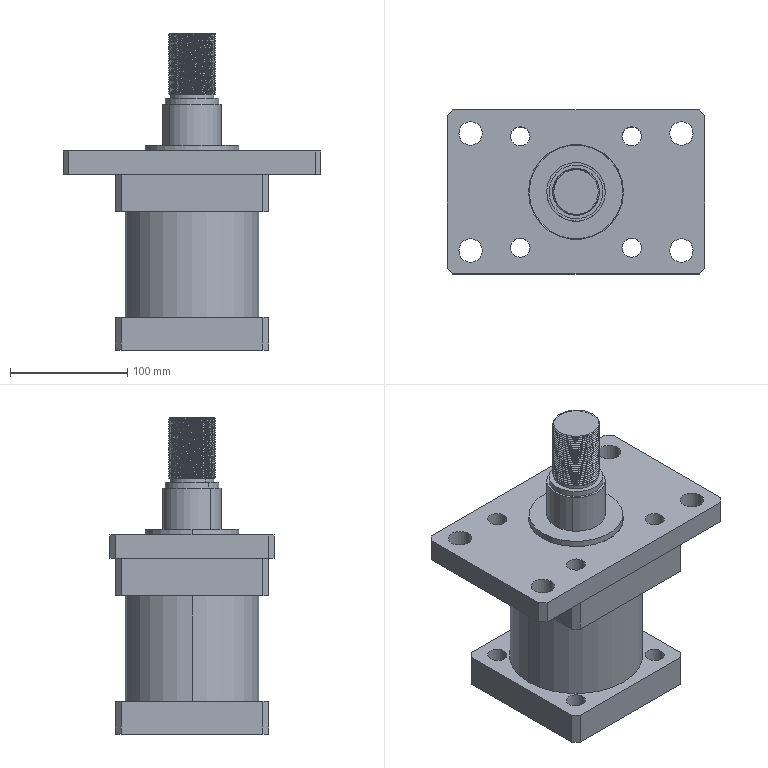Part | SolidWorks | 3 solids | 157 faces | box 220 x 140 x 270 mm | volume 2443488 mm3 | cylinder 107 | plane 39 | cone 8 | spline 3 | commonest cylinder face diameters 40 x53 16.5 x24 20 x8 11.8 x4 50 x4 80 x4